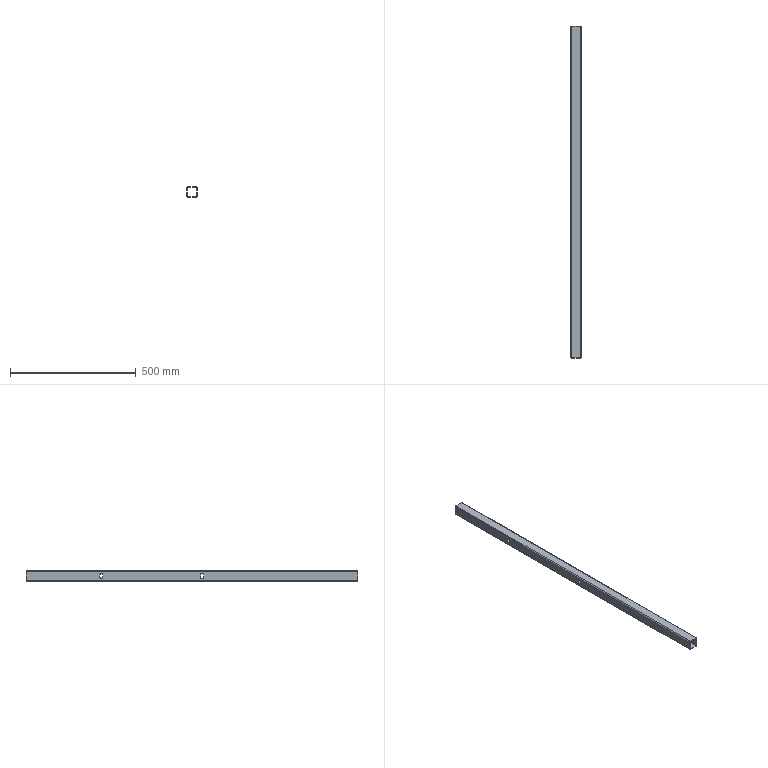Part | STEP file | 粉仓楼梯通道护栏立柱2-1主体_Default<As Machined> | 1 solid | 38 faces | box 40 x 1320 x 40 mm | volume 385818 mm3 | cylinder 20 | plane 18 | commonest cylinder face diameters 12 x12 4 x4 8 x4